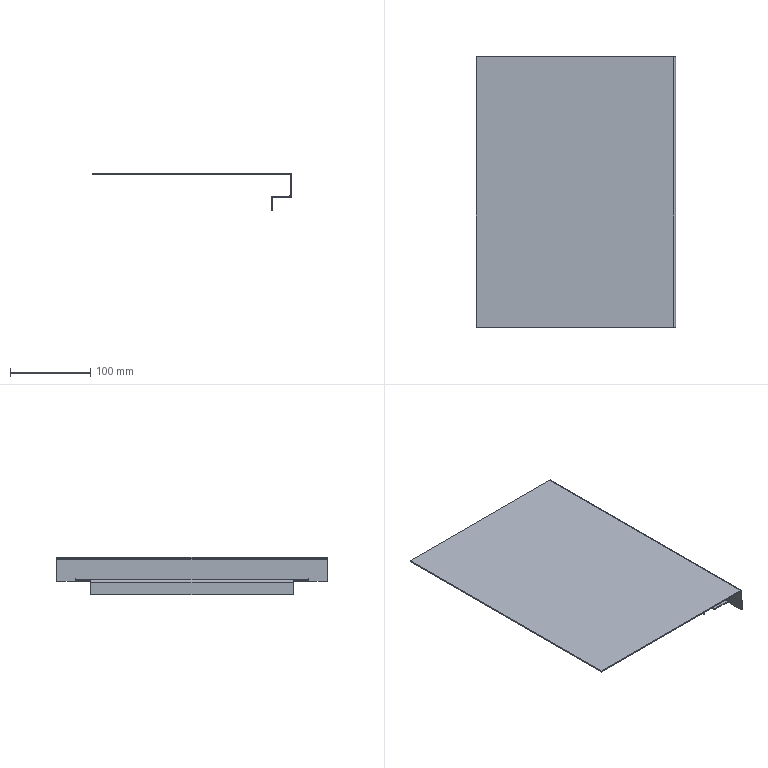Part | SolidWorks | features EdgeFlange 3, FlatPattern 1, SMBaseFlange 1, SheetMetal 1 | 1 solid | 46 faces | box 248.5 x 337 x 47 mm | volume 155691 mm3 | plane 40 | cylinder 6 | commonest cylinder face diameters 2 x3 5 x3
STEP:
#1=CARTESIAN_POINT('',(226.75,295.75,-30.));
#2=VERTEX_POINT('',#1);
#3=CARTESIAN_POINT('',(226.75,295.,-30.));
#4=VERTEX_POINT('',#3);
#5=CARTESIAN_POINT('',(226.75,295.75,-30.));
#6=DIRECTION('',(0.,-1.,0.));
#7=VECTOR('',#6,1000.);
#8=LINE('',#5,#7);
#9=EDGE_CURVE('',#2,#4,#8,.T.);
#10=ORIENTED_EDGE('',*,*,#9,.F.);
#11=CARTESIAN_POINT('',(223.5,295.75,-30.));
#12=VERTEX_POINT('',#11);
#13=CARTESIAN_POINT('',(223.5,295.75,-30.));
#14=DIRECTION('',(1.,0.,0.));
#15=VECTOR('',#14,1000.);
#16=LINE('',#13,#15);
#17=EDGE_CURVE('',#12,#2,#16,.T.);
#18=ORIENTED_EDGE('',*,*,#17,.F.);
#19=CARTESIAN_POINT('',(223.5,313.5,-30.));
#20=VERTEX_POINT('',#19);
#21=CARTESIAN_POINT('',(223.5,23.5,-30.));
#22=DIRECTION('',(0.,-1.,0.));
#23=VECTOR('',#22,1000.);
#24=LINE('',#21,#23);
#25=EDGE_CURVE('',#20,#12,#24,.T.);
#26=ORIENTED_EDGE('',*,*,#25,.F.);
#27=CARTESIAN_POINT('',(246.,313.5,-30.));
#28=VERTEX_POINT('',#27);
#29=CARTESIAN_POINT('',(223.5,313.5,-30.));
#30=DIRECTION('',(-1.,0.,0.));
#31=VECTOR('',#30,1000.);
#32=LINE('',#29,#31);
#33=EDGE_CURVE('',#28,#20,#32,.T.);
#34=ORIENTED_EDGE('',*,*,#33,.F.);
#35=CARTESIAN_POINT('',(246.,23.5,-30.));
#36=VERTEX_POINT('',#35);
#37=CARTESIAN_POINT('',(246.,0.,-30.));
#38=DIRECTION('',(0.,-1.,0.));
#39=VECTOR('',#38,1000.);
#40=LINE('',#37,#39);
#41=EDGE_CURVE('',#28,#36,#40,.T.);
#42=ORIENTED_EDGE('',*,*,#41,.T.);
#43=CARTESIAN_POINT('',(223.5,23.5,-30.));
#44=VERTEX_POINT('',#43);
#45=CARTESIAN_POINT('',(247.,23.5,-30.));
#46=DIRECTION('',(1.,0.,0.));
#47=VECTOR('',#46,1000.);
#48=LINE('',#45,#47);
#49=EDGE_CURVE('',#44,#36,#48,.T.);
#50=ORIENTED_EDGE('',*,*,#49,.F.);
#51=CARTESIAN_POINT('',(223.5,41.25,-30.));
#52=VERTEX_POINT('',#51);
#53=CARTESIAN_POINT('',(223.5,23.5,-30.));
#54=DIRECTION('',(0.,-1.,0.));
#55=VECTOR('',#54,1000.);
#56=LINE('',#53,#55);
#57=EDGE_CURVE('',#52,#44,#56,.T.);
#58=ORIENTED_EDGE('',*,*,#57,.F.);
#59=CARTESIAN_POINT('',(226.75,41.25,-30.));
#60=VERTEX_POINT('',#59);
#61=CARTESIAN_POINT('',(226.75,41.25,-30.));
#62=DIRECTION('',(-1.,0.,0.));
#63=VECTOR('',#62,1000.);
#64=LINE('',#61,#63);
#65=EDGE_CURVE('',#60,#52,#64,.T.);
#66=ORIENTED_EDGE('',*,*,#65,.F.);
#67=CARTESIAN_POINT('',(226.75,42.,-30.));
#68=VERTEX_POINT('',#67);
#69=CARTESIAN_POINT('',(226.75,42.,-30.));
#70=DIRECTION('',(0.,-1.,0.));
#71=VECTOR('',#70,1000.);
#72=LINE('',#69,#71);
#73=EDGE_CURVE('',#68,#60,#72,.T.);
#74=ORIENTED_EDGE('',*,*,#73,.F.);
#75=CARTESIAN_POINT('',(226.,42.,-30.));
#76=VERTEX_POINT('',#75);
#77=CARTESIAN_POINT('',(226.,42.,-30.));
#78=DIRECTION('',(1.,0.,0.));
#79=VECTOR('',#78,1000.);
#80=LINE('',#77,#79);
#81=EDGE_CURVE('',#76,#68,#80,.T.);
#82=ORIENTED_EDGE('',*,*,#81,.F.);
#83=CARTESIAN_POINT('',(226.,295.,-30.));
#84=VERTEX_POINT('',#83);
#85=CARTESIAN_POINT('',(226.,295.,-30.));
#86=DIRECTION('',(0.,-1.,0.));
#87=VECTOR('',#86,1000.);
#88=LINE('',#85,#87);
#89=EDGE_CURVE('',#84,#76,#88,.T.);
#90=ORIENTED_EDGE('',*,*,#89,.F.);
#91=CARTESIAN_POINT('',(226.75,295.,-30.));
#92=DIRECTION('',(-1.,0.,0.));
#93=VECTOR('',#92,1000.);
#94=LINE('',#91,#93);
#95=EDGE_CURVE('',#4,#84,#94,.T.);
#96=ORIENTED_EDGE('',*,*,#95,.F.);
#97=EDGE_LOOP('',(#10,#18,#26,#34,#42,#50,#58,#66,#74,#82,#90,#96));
#98=FACE_OUTER_BOUND('',#97,.T.);
#99=CARTESIAN_POINT('',(0.,0.,-30.));
#100=DIRECTION('',(0.,0.,-1.));
#101=DIRECTION('',(-1.,0.,0.));
#102=AXIS2_PLACEMENT_3D('',#99,#100,#101);
#103=PLANE('',#102);
#104=ADVANCED_FACE('',(#98),#103,.T.);
#105=CARTESIAN_POINT('',(226.75,295.75,-28.5));
#106=VERTEX_POINT('',#105);
#107=CARTESIAN_POINT('',(223.5,295.75,-28.5));
#108=VERTEX_POINT('',#107);
#109=CARTESIAN_POINT('',(0.,295.75,-28.5));
#110=DIRECTION('',(-1.,0.,0.));
#111=VECTOR('',#110,1000.);
#112=LINE('',#109,#111);
#113=EDGE_CURVE('',#106,#108,#112,.T.);
#114=ORIENTED_EDGE('',*,*,#113,.F.);
#115=CARTESIAN_POINT('',(226.75,295.,-28.5));
#116=VERTEX_POINT('',#115);
#117=CARTESIAN_POINT('',(226.75,0.,-28.5));
#118=DIRECTION('',(0.,1.,0.));
#119=VECTOR('',#118,1000.);
#120=LINE('',#117,#119);
#121=EDGE_CURVE('',#116,#106,#120,.T.);
#122=ORIENTED_EDGE('',*,*,#121,.F.);
#123=CARTESIAN_POINT('',(226.,295.,-28.5));
#124=VERTEX_POINT('',#123);
#125=CARTESIAN_POINT('',(0.,295.,-28.5));
#126=DIRECTION('',(1.,0.,0.));
#127=VECTOR('',#126,1000.);
#128=LINE('',#125,#127);
#129=EDGE_CURVE('',#124,#116,#128,.T.);
#130=ORIENTED_EDGE('',*,*,#129,.F.);
#131=CARTESIAN_POINT('',(226.,42.,-28.5));
#132=VERTEX_POINT('',#131);
#133=CARTESIAN_POINT('',(226.,295.,-28.5));
#134=DIRECTION('',(0.,-1.,0.));
#135=VECTOR('',#134,1000.);
#136=LINE('',#133,#135);
#137=EDGE_CURVE('',#124,#132,#136,.T.);
#138=ORIENTED_EDGE('',*,*,#137,.T.);
#139=CARTESIAN_POINT('',(226.75,42.,-28.5));
#140=VERTEX_POINT('',#139);
#141=CARTESIAN_POINT('',(0.,42.,-28.5));
#142=DIRECTION('',(-1.,0.,0.));
#143=VECTOR('',#142,1000.);
#144=LINE('',#141,#143);
#145=EDGE_CURVE('',#140,#132,#144,.T.);
#146=ORIENTED_EDGE('',*,*,#145,.F.);
#147=CARTESIAN_POINT('',(226.75,41.25,-28.5));
#148=VERTEX_POINT('',#147);
#149=CARTESIAN_POINT('',(226.75,0.,-28.5));
#150=DIRECTION('',(0.,1.,0.));
#151=VECTOR('',#150,1000.);
#152=LINE('',#149,#151);
#153=EDGE_CURVE('',#148,#140,#152,.T.);
#154=ORIENTED_EDGE('',*,*,#153,.F.);
#155=CARTESIAN_POINT('',(223.5,41.25,-28.5));
#156=VERTEX_POINT('',#155);
#157=CARTESIAN_POINT('',(0.,41.25,-28.5));
#158=DIRECTION('',(1.,0.,0.));
#159=VECTOR('',#158,1000.);
#160=LINE('',#157,#159);
#161=EDGE_CURVE('',#156,#148,#160,.T.);
#162=ORIENTED_EDGE('',*,*,#161,.F.);
#163=CARTESIAN_POINT('',(223.5,23.5,-28.5));
#164=VERTEX_POINT('',#163);
#165=CARTESIAN_POINT('',(223.5,0.,-28.5));
#166=DIRECTION('',(0.,-1.,0.));
#167=VECTOR('',#166,1000.);
#168=LINE('',#165,#167);
#169=EDGE_CURVE('',#156,#164,#168,.T.);
#170=ORIENTED_EDGE('',*,*,#169,.T.);
#171=CARTESIAN_POINT('',(246.,23.5,-28.5));
#172=VERTEX_POINT('',#171);
#173=CARTESIAN_POINT('',(0.,23.5,-28.5));
#174=DIRECTION('',(1.,0.,0.));
#175=VECTOR('',#174,1000.);
#176=LINE('',#173,#175);
#177=EDGE_CURVE('',#164,#172,#176,.T.);
#178=ORIENTED_EDGE('',*,*,#177,.T.);
#179=CARTESIAN_POINT('',(246.,313.5,-28.5));
#180=VERTEX_POINT('',#179);
#181=CARTESIAN_POINT('',(246.,313.5,-28.5));
#182=DIRECTION('',(0.,-1.,0.));
#183=VECTOR('',#182,1000.);
#184=LINE('',#181,#183);
#185=EDGE_CURVE('',#180,#172,#184,.T.);
#186=ORIENTED_EDGE('',*,*,#185,.F.);
#187=CARTESIAN_POINT('',(223.5,313.5,-28.5));
#188=VERTEX_POINT('',#187);
#189=CARTESIAN_POINT('',(0.,313.5,-28.5));
#190=DIRECTION('',(-1.,0.,0.));
#191=VECTOR('',#190,1000.);
#192=LINE('',#189,#191);
#193=EDGE_CURVE('',#180,#188,#192,.T.);
#194=ORIENTED_EDGE('',*,*,#193,.T.);
#195=CARTESIAN_POINT('',(223.5,0.,-28.5));
#196=DIRECTION('',(0.,-1.,0.));
#197=VECTOR('',#196,1000.);
#198=LINE('',#195,#197);
#199=EDGE_CURVE('',#188,#108,#198,.T.);
#200=ORIENTED_EDGE('',*,*,#199,.T.);
#201=EDGE_LOOP('',(#114,#122,#130,#138,#146,#154,#162,#170,#178,#186,#194,#200));
#202=FACE_OUTER_BOUND('',#201,.T.);
#203=CARTESIAN_POINT('',(0.,0.,-28.5));
#204=DIRECTION('',(0.,0.,-1.));
#205=DIRECTION('',(-1.,0.,0.));
#206=AXIS2_PLACEMENT_3D('',#203,#204,#205);
#207=PLANE('',#206);
#208=ADVANCED_FACE('',(#202),#207,.F.);
#209=ORIENTED_EDGE('',*,*,#25,.T.);
#210=CARTESIAN_POINT('',(223.5,295.75,-30.));
#211=DIRECTION('',(0.,0.,1.));
#212=VECTOR('',#211,1000.);
#213=LINE('',#210,#212);
#214=EDGE_CURVE('',#12,#108,#213,.T.);
#215=ORIENTED_EDGE('',*,*,#214,.T.);
#216=ORIENTED_EDGE('',*,*,#199,.F.);
#217=CARTESIAN_POINT('',(223.5,313.5,-30.));
#218=DIRECTION('',(0.,0.,1.));
#219=VECTOR('',#218,1000.);
#220=LINE('',#217,#219);
#221=EDGE_CURVE('',#20,#188,#220,.T.);
#222=ORIENTED_EDGE('',*,*,#221,.F.);
#223=EDGE_LOOP('',(#209,#215,#216,#222));
#224=FACE_OUTER_BOUND('',#223,.T.);
#225=CARTESIAN_POINT('',(223.5,23.5,-30.));
#226=DIRECTION('',(-1.,0.,0.));
#227=DIRECTION('',(0.,0.,1.));
#228=AXIS2_PLACEMENT_3D('',#225,#226,#227);
#229=PLANE('',#228);
#230=ADVANCED_FACE('',(#224),#229,.T.);
#231=ORIENTED_EDGE('',*,*,#169,.F.);
#232=CARTESIAN_POINT('',(223.5,41.25,-30.));
#233=DIRECTION('',(0.,0.,1.));
#234=VECTOR('',#233,1000.);
#235=LINE('',#232,#234);
#236=EDGE_CURVE('',#52,#156,#235,.T.);
#237=ORIENTED_EDGE('',*,*,#236,.F.);
#238=ORIENTED_EDGE('',*,*,#57,.T.);
#239=CARTESIAN_POINT('',(223.5,23.5,-30.));
#240=DIRECTION('',(0.,0.,1.));
#241=VECTOR('',#240,1000.);
#242=LINE('',#239,#241);
#243=EDGE_CURVE('',#44,#164,#242,.T.);
#244=ORIENTED_EDGE('',*,*,#243,.T.);
#245=EDGE_LOOP('',(#231,#237,#238,#244));
#246=FACE_OUTER_BOUND('',#245,.T.);
#247=CARTESIAN_POINT('',(223.5,23.5,-30.));
#248=DIRECTION('',(-1.,0.,0.));
#249=DIRECTION('',(0.,0.,1.));
#250=AXIS2_PLACEMENT_3D('',#247,#248,#249);
#251=PLANE('',#250);
#252=ADVANCED_FACE('',(#246),#251,.T.);
#253=CARTESIAN_POINT('',(248.5,22.75,-30.));
#254=VERTEX_POINT('',#253);
#255=CARTESIAN_POINT('',(248.5,0.,-30.));
#256=VERTEX_POINT('',#255);
#257=CARTESIAN_POINT('',(248.5,0.,-30.));
#258=DIRECTION('',(0.,-1.,0.));
#259=VECTOR('',#258,1000.);
#260=LINE('',#257,#259);
#261=EDGE_CURVE('',#254,#256,#260,.T.);
#262=ORIENTED_EDGE('',*,*,#261,.F.);
#263=CARTESIAN_POINT('',(248.5,22.75,-26.75));
#264=VERTEX_POINT('',#263);
#265=CARTESIAN_POINT('',(248.5,22.75,0.));
#266=DIRECTION('',(0.,0.,1.));
#267=VECTOR('',#266,1000.);
#268=LINE('',#265,#267);
#269=EDGE_CURVE('',#254,#264,#268,.T.);
#270=ORIENTED_EDGE('',*,*,#269,.T.);
#271=CARTESIAN_POINT('',(248.5,23.5,-26.75));
#272=VERTEX_POINT('',#271);
#273=CARTESIAN_POINT('',(248.5,0.,-26.75));
#274=DIRECTION('',(0.,1.,0.));
#275=VECTOR('',#274,1000.);
#276=LINE('',#273,#275);
#277=EDGE_CURVE('',#264,#272,#276,.T.);
#278=ORIENTED_EDGE('',*,*,#277,.T.);
#279=CARTESIAN_POINT('',(248.5,23.5,-27.5));
#280=VERTEX_POINT('',#279);
#281=CARTESIAN_POINT('',(248.5,23.5,0.));
#282=DIRECTION('',(0.,0.,-1.));
#283=VECTOR('',#282,1000.);
#284=LINE('',#281,#283);
#285=EDGE_CURVE('',#272,#280,#284,.T.);
#286=ORIENTED_EDGE('',*,*,#285,.T.);
#287=CARTESIAN_POINT('',(248.5,313.5,-27.5));
#288=VERTEX_POINT('',#287);
#289=CARTESIAN_POINT('',(248.5,23.5,-27.5));
#290=DIRECTION('',(0.,1.,0.));
#291=VECTOR('',#290,1000.);
#292=LINE('',#289,#291);
#293=EDGE_CURVE('',#280,#288,#292,.T.);
#294=ORIENTED_EDGE('',*,*,#293,.T.);
#295=CARTESIAN_POINT('',(248.5,313.5,-26.75));
#296=VERTEX_POINT('',#295);
#297=CARTESIAN_POINT('',(248.5,313.5,0.));
#298=DIRECTION('',(0.,0.,1.));
#299=VECTOR('',#298,1000.);
#300=LINE('',#297,#299);
#301=EDGE_CURVE('',#288,#296,#300,.T.);
#302=ORIENTED_EDGE('',*,*,#301,.T.);
#303=CARTESIAN_POINT('',(248.5,314.25,-26.75));
#304=VERTEX_POINT('',#303);
#305=CARTESIAN_POINT('',(248.5,0.,-26.75));
#306=DIRECTION('',(0.,1.,0.));
#307=VECTOR('',#306,1000.);
#308=LINE('',#305,#307);
#309=EDGE_CURVE('',#296,#304,#308,.T.);
#310=ORIENTED_EDGE('',*,*,#309,.T.);
#311=CARTESIAN_POINT('',(248.5,314.25,-30.));
#312=VERTEX_POINT('',#311);
#313=CARTESIAN_POINT('',(248.5,314.25,0.));
#314=DIRECTION('',(0.,0.,-1.));
#315=VECTOR('',#314,1000.);
#316=LINE('',#313,#315);
#317=EDGE_CURVE('',#304,#312,#316,.T.);
#318=ORIENTED_EDGE('',*,*,#317,.T.);
#319=CARTESIAN_POINT('',(248.5,337.,-30.));
#320=VERTEX_POINT('',#319);
#321=CARTESIAN_POINT('',(248.5,0.,-30.));
#322=DIRECTION('',(0.,-1.,0.));
#323=VECTOR('',#322,1000.);
#324=LINE('',#321,#323);
#325=EDGE_CURVE('',#320,#312,#324,.T.);
#326=ORIENTED_EDGE('',*,*,#325,.F.);
#327=CARTESIAN_POINT('',(248.5,337.,-2.5));
#328=VERTEX_POINT('',#327);
#329=CARTESIAN_POINT('',(248.5,337.,-30.));
#330=DIRECTION('',(0.,0.,-1.));
#331=VECTOR('',#330,1000.);
#332=LINE('',#329,#331);
#333=EDGE_CURVE('',#328,#320,#332,.T.);
#334=ORIENTED_EDGE('',*,*,#333,.F.);
#335=CARTESIAN_POINT('',(248.5,0.,-2.5));
#336=VERTEX_POINT('',#335);
#337=CARTESIAN_POINT('',(248.5,0.,-2.5));
#338=DIRECTION('',(0.,-1.,0.));
#339=VECTOR('',#338,1000.);
#340=LINE('',#337,#339);
#341=EDGE_CURVE('',#328,#336,#340,.T.);
#342=ORIENTED_EDGE('',*,*,#341,.T.);
#343=CARTESIAN_POINT('',(248.5,0.,-1.5));
#344=DIRECTION('',(0.,0.,1.));
#345=VECTOR('',#344,1000.);
#346=LINE('',#343,#345);
#347=EDGE_CURVE('',#256,#336,#346,.T.);
#348=ORIENTED_EDGE('',*,*,#347,.F.);
#349=EDGE_LOOP('',(#262,#270,#278,#286,#294,#302,#310,#318,#326,#334,#342,#348));
#350=FACE_OUTER_BOUND('',#349,.T.);
#351=CARTESIAN_POINT('',(248.5,0.,0.));
#352=DIRECTION('',(1.,0.,0.));
#353=DIRECTION('',(0.,0.,-1.));
#354=AXIS2_PLACEMENT_3D('',#351,#352,#353);
#355=PLANE('',#354);
#356=ADVANCED_FACE('',(#350),#355,.T.);
#357=CARTESIAN_POINT('',(247.,22.75,-30.));
#358=VERTEX_POINT('',#357);
#359=CARTESIAN_POINT('',(247.,22.75,-26.75));
#360=VERTEX_POINT('',#359);
#361=CARTESIAN_POINT('',(247.,22.75,-30.));
#362=DIRECTION('',(0.,0.,1.));
#363=VECTOR('',#362,1000.);
#364=LINE('',#361,#363);
#365=EDGE_CURVE('',#358,#360,#364,.T.);
#366=ORIENTED_EDGE('',*,*,#365,.F.);
#367=CARTESIAN_POINT('',(247.,0.,-30.));
#368=VERTEX_POINT('',#367);
#369=CARTESIAN_POINT('',(247.,0.,-30.));
#370=DIRECTION('',(0.,-1.,0.));
#371=VECTOR('',#370,1000.);
#372=LINE('',#369,#371);
#373=EDGE_CURVE('',#358,#368,#372,.T.);
#374=ORIENTED_EDGE('',*,*,#373,.T.);
#375=CARTESIAN_POINT('',(247.,0.,-2.5));
#376=VERTEX_POINT('',#375);
#377=CARTESIAN_POINT('',(247.,0.,0.));
#378=DIRECTION('',(0.,0.,1.));
#379=VECTOR('',#378,1000.);
#380=LINE('',#377,#379);
#381=EDGE_CURVE('',#368,#376,#380,.T.);
#382=ORIENTED_EDGE('',*,*,#381,.T.);
#383=CARTESIAN_POINT('',(247.,337.,-2.5));
#384=VERTEX_POINT('',#383);
#385=CARTESIAN_POINT('',(247.,337.,-2.5));
#386=DIRECTION('',(0.,-1.,0.));
#387=VECTOR('',#386,1000.);
#388=LINE('',#385,#387);
#389=EDGE_CURVE('',#384,#376,#388,.T.);
#390=ORIENTED_EDGE('',*,*,#389,.F.);
#391=CARTESIAN_POINT('',(247.,337.,-30.));
#392=VERTEX_POINT('',#391);
#393=CARTESIAN_POINT('',(247.,337.,0.));
#394=DIRECTION('',(0.,0.,-1.));
#395=VECTOR('',#394,1000.);
#396=LINE('',#393,#395);
#397=EDGE_CURVE('',#384,#392,#396,.T.);
#398=ORIENTED_EDGE('',*,*,#397,.T.);
#399=CARTESIAN_POINT('',(247.,314.25,-30.));
#400=VERTEX_POINT('',#399);
#401=CARTESIAN_POINT('',(247.,0.,-30.));
#402=DIRECTION('',(0.,-1.,0.));
#403=VECTOR('',#402,1000.);
#404=LINE('',#401,#403);
#405=EDGE_CURVE('',#392,#400,#404,.T.);
#406=ORIENTED_EDGE('',*,*,#405,.T.);
#407=CARTESIAN_POINT('',(247.,314.25,-26.75));
#408=VERTEX_POINT('',#407);
#409=CARTESIAN_POINT('',(247.,314.25,-26.75));
#410=DIRECTION('',(0.,0.,-1.));
#411=VECTOR('',#410,1000.);
#412=LINE('',#409,#411);
#413=EDGE_CURVE('',#408,#400,#412,.T.);
#414=ORIENTED_EDGE('',*,*,#413,.F.);
#415=CARTESIAN_POINT('',(247.,313.5,-26.75));
#416=VERTEX_POINT('',#415);
#417=CARTESIAN_POINT('',(247.,313.5,-26.75));
#418=DIRECTION('',(0.,1.,0.));
#419=VECTOR('',#418,1000.);
#420=LINE('',#417,#419);
#421=EDGE_CURVE('',#416,#408,#420,.T.);
#422=ORIENTED_EDGE('',*,*,#421,.F.);
#423=CARTESIAN_POINT('',(247.,313.5,-27.5));
#424=VERTEX_POINT('',#423);
#425=CARTESIAN_POINT('',(247.,313.5,-27.5));
#426=DIRECTION('',(0.,0.,1.));
#427=VECTOR('',#426,1000.);
#428=LINE('',#425,#427);
#429=EDGE_CURVE('',#424,#416,#428,.T.);
#430=ORIENTED_EDGE('',*,*,#429,.F.);
#431=CARTESIAN_POINT('',(247.,23.5,-27.5));
#432=VERTEX_POINT('',#431);
#433=CARTESIAN_POINT('',(247.,23.5,-27.5));
#434=DIRECTION('',(0.,1.,0.));
#435=VECTOR('',#434,1000.);
#436=LINE('',#433,#435);
#437=EDGE_CURVE('',#432,#424,#436,.T.);
#438=ORIENTED_EDGE('',*,*,#437,.F.);
#439=CARTESIAN_POINT('',(247.,23.5,-26.75));
#440=VERTEX_POINT('',#439);
#441=CARTESIAN_POINT('',(247.,23.5,-26.75));
#442=DIRECTION('',(0.,0.,-1.));
#443=VECTOR('',#442,1000.);
#444=LINE('',#441,#443);
#445=EDGE_CURVE('',#440,#432,#444,.T.);
#446=ORIENTED_EDGE('',*,*,#445,.F.);
#447=CARTESIAN_POINT('',(247.,22.75,-26.75));
#448=DIRECTION('',(0.,1.,0.));
#449=VECTOR('',#448,1000.);
#450=LINE('',#447,#449);
#451=EDGE_CURVE('',#360,#440,#450,.T.);
#452=ORIENTED_EDGE('',*,*,#451,.F.);
#453=EDGE_LOOP('',(#366,#374,#382,#390,#398,#406,#414,#422,#430,#438,#446,#452));
#454=FACE_OUTER_BOUND('',#453,.T.);
#455=CARTESIAN_POINT('',(247.,0.,0.));
#456=DIRECTION('',(1.,0.,0.));
#457=DIRECTION('',(0.,0.,-1.));
#458=AXIS2_PLACEMENT_3D('',#455,#456,#457);
#459=PLANE('',#458);
#460=ADVANCED_FACE('',(#454),#459,.F.);
#461=ORIENTED_EDGE('',*,*,#373,.F.);
#462=CARTESIAN_POINT('',(247.,22.75,-30.));
#463=DIRECTION('',(1.,0.,0.));
#464=VECTOR('',#463,1000.);
#465=LINE('',#462,#464);
#466=EDGE_CURVE('',#358,#254,#465,.T.);
#467=ORIENTED_EDGE('',*,*,#466,.T.);
#468=ORIENTED_EDGE('',*,*,#261,.T.);
#469=CARTESIAN_POINT('',(248.5,0.,-30.));
#470=DIRECTION('',(-1.,0.,0.));
#471=VECTOR('',#470,1000.);
#472=LINE('',#469,#471);
#473=EDGE_CURVE('',#256,#368,#472,.T.);
#474=ORIENTED_EDGE('',*,*,#473,.T.);
#475=EDGE_LOOP('',(#461,#467,#468,#474));
#476=FACE_OUTER_BOUND('',#475,.T.);
#477=CARTESIAN_POINT('',(248.5,0.,-30.));
#478=DIRECTION('',(0.,0.,-1.));
#479=DIRECTION('',(-1.,0.,0.));
#480=AXIS2_PLACEMENT_3D('',#477,#478,#479);
#481=PLANE('',#480);
#482=ADVANCED_FACE('',(#476),#481,.T.);
#483=ORIENTED_EDGE('',*,*,#325,.T.);
#484=CARTESIAN_POINT('',(247.,314.25,-30.));
#485=DIRECTION('',(1.,0.,0.));
#486=VECTOR('',#485,1000.);
#487=LINE('',#484,#486);
#488=EDGE_CURVE('',#400,#312,#487,.T.);
#489=ORIENTED_EDGE('',*,*,#488,.F.);
#490=ORIENTED_EDGE('',*,*,#405,.F.);
#491=CARTESIAN_POINT('',(248.5,337.,-30.));
#492=DIRECTION('',(-1.,0.,0.));
#493=VECTOR('',#492,1000.);
#494=LINE('',#491,#493);
#495=EDGE_CURVE('',#320,#392,#494,.T.);
#496=ORIENTED_EDGE('',*,*,#495,.F.);
#497=EDGE_LOOP('',(#483,#489,#490,#496));
#498=FACE_OUTER_BOUND('',#497,.T.);
#499=CARTESIAN_POINT('',(248.5,0.,-30.));
#500=DIRECTION('',(0.,0.,-1.));
#501=DIRECTION('',(-1.,0.,0.));
#502=AXIS2_PLACEMENT_3D('',#499,#500,#501);
#503=PLANE('',#502);
#504=ADVANCED_FACE('',(#498),#503,.T.);
#505=CARTESIAN_POINT('',(0.,0.,-1.5));
#506=VERTEX_POINT('',#505);
#507=CARTESIAN_POINT('',(246.,0.,-1.5));
#508=VERTEX_POINT('',#507);
#509=CARTESIAN_POINT('',(0.,0.,-1.5));
#510=DIRECTION('',(1.,0.,0.));
#511=VECTOR('',#510,1000.);
#512=LINE('',#509,#511);
#513=EDGE_CURVE('',#506,#508,#512,.T.);
#514=ORIENTED_EDGE('',*,*,#513,.T.);
#515=CARTESIAN_POINT('',(246.,0.,0.));
#516=VERTEX_POINT('',#515);
#517=CARTESIAN_POINT('',(246.,0.,-1.5));
#518=DIRECTION('',(0.,0.,1.));
#519=VECTOR('',#518,1000.);
#520=LINE('',#517,#519);
#521=EDGE_CURVE('',#508,#516,#520,.T.);
#522=ORIENTED_EDGE('',*,*,#521,.T.);
#523=CARTESIAN_POINT('',(0.,0.,0.));
#524=VERTEX_POINT('',#523);
#525=CARTESIAN_POINT('',(0.,0.,0.));
#526=DIRECTION('',(1.,0.,0.));
#527=VECTOR('',#526,1000.);
#528=LINE('',#525,#527);
#529=EDGE_CURVE('',#524,#516,#528,.T.);
#530=ORIENTED_EDGE('',*,*,#529,.F.);
#531=CARTESIAN_POINT('',(0.,0.,-1.5));
#532=DIRECTION('',(0.,0.,1.));
#533=VECTOR('',#532,1000.);
#534=LINE('',#531,#533);
#535=EDGE_CURVE('',#506,#524,#534,.T.);
#536=ORIENTED_EDGE('',*,*,#535,.F.);
#537=EDGE_LOOP('',(#514,#522,#530,#536));
#538=FACE_OUTER_BOUND('',#537,.T.);
#539=CARTESIAN_POINT('',(0.,0.,-1.5));
#540=DIRECTION('',(0.,-1.,0.));
#541=DIRECTION('',(0.,0.,-1.));
#542=AXIS2_PLACEMENT_3D('',#539,#540,#541);
#543=PLANE('',#542);
#544=ADVANCED_FACE('',(#538),#543,.T.);
#545=CARTESIAN_POINT('',(246.,337.,-1.5));
#546=VERTEX_POINT('',#545);
#547=CARTESIAN_POINT('',(0.,337.,-1.5));
#548=VERTEX_POINT('',#547);
#549=CARTESIAN_POINT('',(0.,337.,-1.5));
#550=DIRECTION('',(-1.,0.,0.));
#551=VECTOR('',#550,1000.);
#552=LINE('',#549,#551);
#553=EDGE_CURVE('',#546,#548,#552,.T.);
#554=ORIENTED_EDGE('',*,*,#553,.F.);
#555=CARTESIAN_POINT('',(246.,0.,-1.5));
#556=DIRECTION('',(0.,1.,0.));
#557=VECTOR('',#556,1000.);
#558=LINE('',#555,#557);
#559=EDGE_CURVE('',#508,#546,#558,.T.);
#560=ORIENTED_EDGE('',*,*,#559,.F.);
#561=ORIENTED_EDGE('',*,*,#513,.F.);
#562=CARTESIAN_POINT('',(0.,0.,-1.5));
#563=DIRECTION('',(0.,-1.,0.));
#564=VECTOR('',#563,1000.);
#565=LINE('',#562,#564);
#566=EDGE_CURVE('',#548,#506,#565,.T.);
#567=ORIENTED_EDGE('',*,*,#566,.F.);
#568=EDGE_LOOP('',(#554,#560,#561,#567));
#569=FACE_OUTER_BOUND('',#568,.T.);
#570=CARTESIAN_POINT('',(0.,0.,-1.5));
#571=DIRECTION('',(0.,0.,-1.));
#572=DIRECTION('',(-1.,0.,0.));
#573=AXIS2_PLACEMENT_3D('',#570,#571,#572);
#574=PLANE('',#573);
#575=ADVANCED_FACE('',(#569),#574,.T.);
#576=CARTESIAN_POINT('',(246.,337.,0.));
#577=VERTEX_POINT('',#576);
#578=CARTESIAN_POINT('',(246.,0.,0.));
#579=DIRECTION('',(0.,1.,0.));
#580=VECTOR('',#579,1000.);
#581=LINE('',#578,#580);
#582=EDGE_CURVE('',#516,#577,#581,.T.);
#583=ORIENTED_EDGE('',*,*,#582,.T.);
#584=CARTESIAN_POINT('',(0.,337.,0.));
#585=VERTEX_POINT('',#584);
#586=CARTESIAN_POINT('',(0.,337.,0.));
#587=DIRECTION('',(-1.,0.,0.));
#588=VECTOR('',#587,1000.);
#589=LINE('',#586,#588);
#590=EDGE_CURVE('',#577,#585,#589,.T.);
#591=ORIENTED_EDGE('',*,*,#590,.T.);
#592=CARTESIAN_POINT('',(0.,0.,0.));
#593=DIRECTION('',(0.,-1.,0.));
#594=VECTOR('',#593,1000.);
#595=LINE('',#592,#594);
#596=EDGE_CURVE('',#585,#524,#595,.T.);
#597=ORIENTED_EDGE('',*,*,#596,.T.);
#598=ORIENTED_EDGE('',*,*,#529,.T.);
#599=EDGE_LOOP('',(#583,#591,#597,#598));
#600=FACE_OUTER_BOUND('',#599,.T.);
#601=CARTESIAN_POINT('',(0.,0.,0.));
#602=DIRECTION('',(0.,0.,-1.));
#603=DIRECTION('',(-1.,0.,0.));
#604=AXIS2_PLACEMENT_3D('',#601,#602,#603);
#605=PLANE('',#604);
#606=ADVANCED_FACE('',(#600),#605,.F.);
#607=ORIENTED_EDGE('',*,*,#596,.F.);
#608=CARTESIAN_POINT('',(0.,337.,-1.5));
#609=DIRECTION('',(0.,0.,1.));
#610=VECTOR('',#609,1000.);
#611=LINE('',#608,#610);
#612=EDGE_CURVE('',#548,#585,#611,.T.);
#613=ORIENTED_EDGE('',*,*,#612,.F.);
#614=ORIENTED_EDGE('',*,*,#566,.T.);
#615=ORIENTED_EDGE('',*,*,#535,.T.);
#616=EDGE_LOOP('',(#607,#613,#614,#615));
#617=FACE_OUTER_BOUND('',#616,.T.);
#618=CARTESIAN_POINT('',(0.,0.,-1.5));
#619=DIRECTION('',(-1.,0.,0.));
#620=DIRECTION('',(0.,0.,1.));
#621=AXIS2_PLACEMENT_3D('',#618,#619,#620);
#622=PLANE('',#621);
#623=ADVANCED_FACE('',(#617),#622,.T.);
#624=CARTESIAN_POINT('',(246.,337.,-1.5));
#625=DIRECTION('',(0.,0.,1.));
#626=VECTOR('',#625,1000.);
#627=LINE('',#624,#626);
#628=EDGE_CURVE('',#546,#577,#627,.T.);
#629=ORIENTED_EDGE('',*,*,#628,.F.);
#630=ORIENTED_EDGE('',*,*,#553,.T.);
#631=ORIENTED_EDGE('',*,*,#612,.T.);
#632=ORIENTED_EDGE('',*,*,#590,.F.);
#633=EDGE_LOOP('',(#629,#630,#631,#632));
#634=FACE_OUTER_BOUND('',#633,.T.);
#635=CARTESIAN_POINT('',(0.,337.,-1.5));
#636=DIRECTION('',(0.,1.,0.));
#637=DIRECTION('',(0.,0.,1.));
#638=AXIS2_PLACEMENT_3D('',#635,#636,#637);
#639=PLANE('',#638);
#640=ADVANCED_FACE('',(#634),#639,.T.);
#641=CARTESIAN_POINT('',(248.5,337.,-2.5));
#642=DIRECTION('',(1.,0.,0.));
#643=VECTOR('',#642,1000.);
#644=LINE('',#641,#643);
#645=EDGE_CURVE('',#384,#328,#644,.T.);
#646=ORIENTED_EDGE('',*,*,#645,.F.);
#647=CARTESIAN_POINT('',(246.,337.,-2.5));
#648=DIRECTION('',(0.,1.,0.));
#649=DIRECTION('',(0.,0.,-1.));
#650=AXIS2_PLACEMENT_3D('',#647,#648,#649);
#651=CIRCLE('',#650,1.);
#652=EDGE_CURVE('',#546,#384,#651,.T.);
#653=ORIENTED_EDGE('',*,*,#652,.F.);
#654=ORIENTED_EDGE('',*,*,#628,.T.);
#655=CARTESIAN_POINT('',(246.,337.,-2.5));
#656=DIRECTION('',(0.,1.,0.));
#657=DIRECTION('',(0.,0.,-1.));
#658=AXIS2_PLACEMENT_3D('',#655,#656,#657);
#659=CIRCLE('',#658,2.5);
#660=EDGE_CURVE('',#577,#328,#659,.T.);
#661=ORIENTED_EDGE('',*,*,#660,.T.);
#662=EDGE_LOOP('',(#646,#653,#654,#661));
#663=FACE_OUTER_BOUND('',#662,.T.);
#664=CARTESIAN_POINT('',(246.,337.,-2.5));
#665=DIRECTION('',(0.,1.,0.));
#666=DIRECTION('',(0.,0.,1.));
#667=AXIS2_PLACEMENT_3D('',#664,#665,#666);
#668=PLANE('',#667);
#669=ADVANCED_FACE('',(#663),#668,.T.);
#670=CARTESIAN_POINT('',(246.,0.,-2.5));
#671=DIRECTION('',(0.,-1.,0.));
#672=DIRECTION('',(0.,0.,-1.));
#673=AXIS2_PLACEMENT_3D('',#670,#671,#672);
#674=CIRCLE('',#673,1.);
#675=EDGE_CURVE('',#376,#508,#674,.T.);
#676=ORIENTED_EDGE('',*,*,#675,.F.);
#677=CARTESIAN_POINT('',(247.,0.,-2.5));
#678=DIRECTION('',(1.,0.,0.));
#679=VECTOR('',#678,1000.);
#680=LINE('',#677,#679);
#681=EDGE_CURVE('',#376,#336,#680,.T.);
#682=ORIENTED_EDGE('',*,*,#681,.T.);
#683=CARTESIAN_POINT('',(246.,0.,-2.5));
#684=DIRECTION('',(0.,-1.,0.));
#685=DIRECTION('',(0.,0.,-1.));
#686=AXIS2_PLACEMENT_3D('',#683,#684,#685);
#687=CIRCLE('',#686,2.5);
#688=EDGE_CURVE('',#336,#516,#687,.T.);
#689=ORIENTED_EDGE('',*,*,#688,.T.);
#690=ORIENTED_EDGE('',*,*,#521,.F.);
#691=EDGE_LOOP('',(#676,#682,#689,#690));
#692=FACE_OUTER_BOUND('',#691,.T.);
#693=CARTESIAN_POINT('',(246.,0.,-2.5));
#694=DIRECTION('',(0.,1.,0.));
#695=DIRECTION('',(0.,0.,1.));
#696=AXIS2_PLACEMENT_3D('',#693,#694,#695);
#697=PLANE('',#696);
#698=ADVANCED_FACE('',(#692),#697,.F.);
#699=ORIENTED_EDGE('',*,*,#582,.F.);
#700=ORIENTED_EDGE('',*,*,#688,.F.);
#701=ORIENTED_EDGE('',*,*,#341,.F.);
#702=ORIENTED_EDGE('',*,*,#660,.F.);
#703=EDGE_LOOP('',(#699,#700,#701,#702));
#704=FACE_OUTER_BOUND('',#703,.T.);
#705=CARTESIAN_POINT('',(246.,0.,-2.5));
#706=DIRECTION('',(0.,-1.,0.));
#707=DIRECTION('',(1.,0.,0.));
#708=AXIS2_PLACEMENT_3D('',#705,#706,#707);
#709=CYLINDRICAL_SURFACE('',#708,2.5);
#710=ADVANCED_FACE('',(#704),#709,.T.);
#711=ORIENTED_EDGE('',*,*,#559,.T.);
#712=ORIENTED_EDGE('',*,*,#652,.T.);
#713=ORIENTED_EDGE('',*,*,#389,.T.);
#714=ORIENTED_EDGE('',*,*,#675,.T.);
#715=EDGE_LOOP('',(#711,#712,#713,#714));
#716=FACE_OUTER_BOUND('',#715,.T.);
#717=CARTESIAN_POINT('',(246.,0.,-2.5));
#718=DIRECTION('',(0.,-1.,0.));
#719=DIRECTION('',(1.,0.,0.));
#720=AXIS2_PLACEMENT_3D('',#717,#718,#719);
#721=CYLINDRICAL_SURFACE('',#720,1.);
#722=ADVANCED_FACE('',(#716),#721,.F.);
#723=ORIENTED_EDGE('',*,*,#347,.T.);
#724=ORIENTED_EDGE('',*,*,#681,.F.);
#725=ORIENTED_EDGE('',*,*,#381,.F.);
#726=ORIENTED_EDGE('',*,*,#473,.F.);
#727=EDGE_LOOP('',(#723,#724,#725,#726));
#728=FACE_OUTER_BOUND('',#727,.T.);
#729=CARTESIAN_POINT('',(248.5,0.,-1.5));
#730=DIRECTION('',(0.,-1.,0.));
#731=DIRECTION('',(0.,0.,-1.));
#732=AXIS2_PLACEMENT_3D('',#729,#730,#731);
#733=PLANE('',#732);
#734=ADVANCED_FACE('',(#728),#733,.T.);
#735=ORIENTED_EDGE('',*,*,#397,.F.);
#736=ORIENTED_EDGE('',*,*,#645,.T.);
#737=ORIENTED_EDGE('',*,*,#333,.T.);
#738=ORIENTED_EDGE('',*,*,#495,.T.);
#739=EDGE_LOOP('',(#735,#736,#737,#738));
#740=FACE_OUTER_BOUND('',#739,.T.);
#741=CARTESIAN_POINT('',(248.5,337.,-30.));
#742=DIRECTION('',(0.,1.,0.));
#743=DIRECTION('',(0.,0.,1.));
#744=AXIS2_PLACEMENT_3D('',#741,#742,#743);
#745=PLANE('',#744);
#746=ADVANCED_FACE('',(#740),#745,.T.);
#747=ORIENTED_EDGE('',*,*,#269,.F.);
#748=ORIENTED_EDGE('',*,*,#466,.F.);
#749=ORIENTED_EDGE('',*,*,#365,.T.);
#750=CARTESIAN_POINT('',(247.,22.75,-26.75));
#751=DIRECTION('',(1.,0.,0.));
#752=VECTOR('',#751,1000.);
#753=LINE('',#750,#752);
#754=EDGE_CURVE('',#360,#264,#753,.T.);
#755=ORIENTED_EDGE('',*,*,#754,.T.);
#756=EDGE_LOOP('',(#747,#748,#749,#755));
#757=FACE_OUTER_BOUND('',#756,.T.);
#758=CARTESIAN_POINT('',(247.,22.75,-30.));
#759=DIRECTION('',(0.,1.,0.));
#760=DIRECTION('',(0.,0.,1.));
#761=AXIS2_PLACEMENT_3D('',#758,#759,#760);
#762=PLANE('',#761);
#763=ADVANCED_FACE('',(#757),#762,.T.);
#764=ORIENTED_EDGE('',*,*,#277,.F.);
#765=ORIENTED_EDGE('',*,*,#754,.F.);
#766=ORIENTED_EDGE('',*,*,#451,.T.);
#767=CARTESIAN_POINT('',(247.,23.5,-26.75));
#768=DIRECTION('',(1.,0.,0.));
#769=VECTOR('',#768,1000.);
#770=LINE('',#767,#769);
#771=EDGE_CURVE('',#440,#272,#770,.T.);
#772=ORIENTED_EDGE('',*,*,#771,.T.);
#773=EDGE_LOOP('',(#764,#765,#766,#772));
#774=FACE_OUTER_BOUND('',#773,.T.);
#775=CARTESIAN_POINT('',(247.,22.75,-26.75));
#776=DIRECTION('',(0.,0.,-1.));
#777=DIRECTION('',(-1.,0.,0.));
#778=AXIS2_PLACEMENT_3D('',#775,#776,#777);
#779=PLANE('',#778);
#780=ADVANCED_FACE('',(#774),#779,.T.);
#781=ORIENTED_EDGE('',*,*,#285,.F.);
#782=ORIENTED_EDGE('',*,*,#771,.F.);
#783=ORIENTED_EDGE('',*,*,#445,.T.);
#784=CARTESIAN_POINT('',(247.,23.5,-27.5));
#785=DIRECTION('',(1.,0.,0.));
#786=VECTOR('',#785,1000.);
#787=LINE('',#784,#786);
#788=EDGE_CURVE('',#432,#280,#787,.T.);
#789=ORIENTED_EDGE('',*,*,#788,.T.);
#790=EDGE_LOOP('',(#781,#782,#783,#789));
#791=FACE_OUTER_BOUND('',#790,.T.);
#792=CARTESIAN_POINT('',(247.,23.5,-26.75));
#793=DIRECTION('',(0.,-1.,0.));
#794=DIRECTION('',(0.,0.,-1.));
#795=AXIS2_PLACEMENT_3D('',#792,#793,#794);
#796=PLANE('',#795);
#797=ADVANCED_FACE('',(#791),#796,.T.);
#798=ORIENTED_EDGE('',*,*,#301,.F.);
#799=CARTESIAN_POINT('',(247.,313.5,-27.5));
#800=DIRECTION('',(1.,0.,0.));
#801=VECTOR('',#800,1000.);
#802=LINE('',#799,#801);
#803=EDGE_CURVE('',#424,#288,#802,.T.);
#804=ORIENTED_EDGE('',*,*,#803,.F.);
#805=ORIENTED_EDGE('',*,*,#429,.T.);
#806=CARTESIAN_POINT('',(247.,313.5,-26.75));
#807=DIRECTION('',(1.,0.,0.));
#808=VECTOR('',#807,1000.);
#809=LINE('',#806,#808);
#810=EDGE_CURVE('',#416,#296,#809,.T.);
#811=ORIENTED_EDGE('',*,*,#810,.T.);
#812=EDGE_LOOP('',(#798,#804,#805,#811));
#813=FACE_OUTER_BOUND('',#812,.T.);
#814=CARTESIAN_POINT('',(247.,313.5,-27.5));
#815=DIRECTION('',(0.,1.,0.));
#816=DIRECTION('',(0.,0.,1.));
#817=AXIS2_PLACEMENT_3D('',#814,#815,#816);
#818=PLANE('',#817);
#819=ADVANCED_FACE('',(#813),#818,.T.);
#820=ORIENTED_EDGE('',*,*,#309,.F.);
#821=ORIENTED_EDGE('',*,*,#810,.F.);
#822=ORIENTED_EDGE('',*,*,#421,.T.);
#823=CARTESIAN_POINT('',(247.,314.25,-26.75));
#824=DIRECTION('',(1.,0.,0.));
#825=VECTOR('',#824,1000.);
#826=LINE('',#823,#825);
#827=EDGE_CURVE('',#408,#304,#826,.T.);
#828=ORIENTED_EDGE('',*,*,#827,.T.);
#829=EDGE_LOOP('',(#820,#821,#822,#828));
#830=FACE_OUTER_BOUND('',#829,.T.);
#831=CARTESIAN_POINT('',(247.,313.5,-26.75));
#832=DIRECTION('',(0.,0.,-1.));
#833=DIRECTION('',(-1.,0.,0.));
#834=AXIS2_PLACEMENT_3D('',#831,#832,#833);
#835=PLANE('',#834);
#836=ADVANCED_FACE('',(#830),#835,.T.);
#837=ORIENTED_EDGE('',*,*,#317,.F.);
#838=ORIENTED_EDGE('',*,*,#827,.F.);
#839=ORIENTED_EDGE('',*,*,#413,.T.);
#840=ORIENTED_EDGE('',*,*,#488,.T.);
#841=EDGE_LOOP('',(#837,#838,#839,#840));
#842=FACE_OUTER_BOUND('',#841,.T.);
#843=CARTESIAN_POINT('',(247.,314.25,-26.75));
#844=DIRECTION('',(0.,-1.,0.));
#845=DIRECTION('',(0.,0.,-1.));
#846=AXIS2_PLACEMENT_3D('',#843,#844,#845);
#847=PLANE('',#846);
#848=ADVANCED_FACE('',(#842),#847,.T.);
#849=CARTESIAN_POINT('',(246.,313.5,-30.));
#850=DIRECTION('',(0.,0.,-1.));
#851=VECTOR('',#850,1000.);
#852=LINE('',#849,#851);
#853=EDGE_CURVE('',#180,#28,#852,.T.);
#854=ORIENTED_EDGE('',*,*,#853,.F.);
#855=CARTESIAN_POINT('',(246.,313.5,-27.5));
#856=DIRECTION('',(0.,1.,0.));
#857=DIRECTION('',(0.,0.,-1.));
#858=AXIS2_PLACEMENT_3D('',#855,#856,#857);
#859=CIRCLE('',#858,1.);
#860=EDGE_CURVE('',#424,#180,#859,.T.);
#861=ORIENTED_EDGE('',*,*,#860,.F.);
#862=ORIENTED_EDGE('',*,*,#803,.T.);
#863=CARTESIAN_POINT('',(246.,313.5,-27.5));
#864=DIRECTION('',(0.,1.,0.));
#865=DIRECTION('',(0.,0.,-1.));
#866=AXIS2_PLACEMENT_3D('',#863,#864,#865);
#867=CIRCLE('',#866,2.5);
#868=EDGE_CURVE('',#288,#28,#867,.T.);
#869=ORIENTED_EDGE('',*,*,#868,.T.);
#870=EDGE_LOOP('',(#854,#861,#862,#869));
#871=FACE_OUTER_BOUND('',#870,.T.);
#872=CARTESIAN_POINT('',(246.,313.5,-27.5));
#873=DIRECTION('',(0.,1.,0.));
#874=DIRECTION('',(0.,0.,1.));
#875=AXIS2_PLACEMENT_3D('',#872,#873,#874);
#876=PLANE('',#875);
#877=ADVANCED_FACE('',(#871),#876,.T.);
#878=CARTESIAN_POINT('',(246.,23.5,-27.5));
#879=DIRECTION('',(0.,-1.,0.));
#880=DIRECTION('',(0.,0.,-1.));
#881=AXIS2_PLACEMENT_3D('',#878,#879,#880);
#882=CIRCLE('',#881,1.);
#883=EDGE_CURVE('',#172,#432,#882,.T.);
#884=ORIENTED_EDGE('',*,*,#883,.F.);
#885=CARTESIAN_POINT('',(246.,23.5,-28.5));
#886=DIRECTION('',(0.,0.,-1.));
#887=VECTOR('',#886,1000.);
#888=LINE('',#885,#887);
#889=EDGE_CURVE('',#172,#36,#888,.T.);
#890=ORIENTED_EDGE('',*,*,#889,.T.);
#891=CARTESIAN_POINT('',(246.,23.5,-27.5));
#892=DIRECTION('',(0.,-1.,0.));
#893=DIRECTION('',(0.,0.,-1.));
#894=AXIS2_PLACEMENT_3D('',#891,#892,#893);
#895=CIRCLE('',#894,2.5);
#896=EDGE_CURVE('',#36,#280,#895,.T.);
#897=ORIENTED_EDGE('',*,*,#896,.T.);
#898=ORIENTED_EDGE('',*,*,#788,.F.);
#899=EDGE_LOOP('',(#884,#890,#897,#898));
#900=FACE_OUTER_BOUND('',#899,.T.);
#901=CARTESIAN_POINT('',(246.,23.5,-27.5));
#902=DIRECTION('',(0.,1.,0.));
#903=DIRECTION('',(0.,0.,1.));
#904=AXIS2_PLACEMENT_3D('',#901,#902,#903);
#905=PLANE('',#904);
#906=ADVANCED_FACE('',(#900),#905,.F.);
#907=ORIENTED_EDGE('',*,*,#293,.F.);
#908=ORIENTED_EDGE('',*,*,#896,.F.);
#909=ORIENTED_EDGE('',*,*,#41,.F.);
#910=ORIENTED_EDGE('',*,*,#868,.F.);
#911=EDGE_LOOP('',(#907,#908,#909,#910));
#912=FACE_OUTER_BOUND('',#911,.T.);
#913=CARTESIAN_POINT('',(246.,23.5,-27.5));
#914=DIRECTION('',(0.,-1.,0.));
#915=DIRECTION('',(0.,0.,-1.));
#916=AXIS2_PLACEMENT_3D('',#913,#914,#915);
#917=CYLINDRICAL_SURFACE('',#916,2.5);
#918=ADVANCED_FACE('',(#912),#917,.T.);
#919=ORIENTED_EDGE('',*,*,#437,.T.);
#920=ORIENTED_EDGE('',*,*,#860,.T.);
#921=ORIENTED_EDGE('',*,*,#185,.T.);
#922=ORIENTED_EDGE('',*,*,#883,.T.);
#923=EDGE_LOOP('',(#919,#920,#921,#922));
#924=FACE_OUTER_BOUND('',#923,.T.);
#925=CARTESIAN_POINT('',(246.,23.5,-27.5));
#926=DIRECTION('',(0.,-1.,0.));
#927=DIRECTION('',(0.,0.,-1.));
#928=AXIS2_PLACEMENT_3D('',#925,#926,#927);
#929=CYLINDRICAL_SURFACE('',#928,1.);
#930=ADVANCED_FACE('',(#924),#929,.F.);
#931=ORIENTED_EDGE('',*,*,#49,.T.);
#932=ORIENTED_EDGE('',*,*,#889,.F.);
#933=ORIENTED_EDGE('',*,*,#177,.F.);
#934=ORIENTED_EDGE('',*,*,#243,.F.);
#935=EDGE_LOOP('',(#931,#932,#933,#934));
#936=FACE_OUTER_BOUND('',#935,.T.);
#937=CARTESIAN_POINT('',(247.,23.5,-30.));
#938=DIRECTION('',(0.,-1.,0.));
#939=DIRECTION('',(1.,0.,0.));
#940=AXIS2_PLACEMENT_3D('',#937,#938,#939);
#941=PLANE('',#940);
#942=ADVANCED_FACE('',(#936),#941,.T.);
#943=ORIENTED_EDGE('',*,*,#193,.F.);
#944=ORIENTED_EDGE('',*,*,#853,.T.);
#945=ORIENTED_EDGE('',*,*,#33,.T.);
#946=ORIENTED_EDGE('',*,*,#221,.T.);
#947=EDGE_LOOP('',(#943,#944,#945,#946));
#948=FACE_OUTER_BOUND('',#947,.T.);
#949=CARTESIAN_POINT('',(223.5,313.5,-30.));
#950=DIRECTION('',(0.,1.,0.));
#951=DIRECTION('',(0.,0.,1.));
#952=AXIS2_PLACEMENT_3D('',#949,#950,#951);
#953=PLANE('',#952);
#954=ADVANCED_FACE('',(#948),#953,.T.);
#955=CARTESIAN_POINT('',(226.75,295.,-30.));
#956=DIRECTION('',(0.,0.,1.));
#957=VECTOR('',#956,1000.);
#958=LINE('',#955,#957);
#959=EDGE_CURVE('',#4,#116,#958,.T.);
#960=ORIENTED_EDGE('',*,*,#959,.T.);
#961=ORIENTED_EDGE('',*,*,#121,.T.);
#962=CARTESIAN_POINT('',(226.75,295.75,-30.));
#963=DIRECTION('',(0.,0.,1.));
#964=VECTOR('',#963,1000.);
#965=LINE('',#962,#964);
#966=EDGE_CURVE('',#2,#106,#965,.T.);
#967=ORIENTED_EDGE('',*,*,#966,.F.);
#968=ORIENTED_EDGE('',*,*,#9,.T.);
#969=EDGE_LOOP('',(#960,#961,#967,#968));
#970=FACE_OUTER_BOUND('',#969,.T.);
#971=CARTESIAN_POINT('',(226.75,295.75,-30.));
#972=DIRECTION('',(-1.,0.,0.));
#973=DIRECTION('',(0.,0.,1.));
#974=AXIS2_PLACEMENT_3D('',#971,#972,#973);
#975=PLANE('',#974);
#976=ADVANCED_FACE('',(#970),#975,.T.);
#977=CARTESIAN_POINT('',(226.,295.,-30.));
#978=DIRECTION('',(0.,0.,1.));
#979=VECTOR('',#978,1000.);
#980=LINE('',#977,#979);
#981=EDGE_CURVE('',#84,#124,#980,.T.);
#982=ORIENTED_EDGE('',*,*,#981,.T.);
#983=ORIENTED_EDGE('',*,*,#129,.T.);
#984=ORIENTED_EDGE('',*,*,#959,.F.);
#985=ORIENTED_EDGE('',*,*,#95,.T.);
#986=EDGE_LOOP('',(#982,#983,#984,#985));
#987=FACE_OUTER_BOUND('',#986,.T.);
#988=CARTESIAN_POINT('',(226.75,295.,-30.));
#989=DIRECTION('',(0.,1.,0.));
#990=DIRECTION('',(0.,0.,1.));
#991=AXIS2_PLACEMENT_3D('',#988,#989,#990);
#992=PLANE('',#991);
#993=ADVANCED_FACE('',(#987),#992,.T.);
#994=CARTESIAN_POINT('',(226.75,42.,-30.));
#995=DIRECTION('',(0.,0.,1.));
#996=VECTOR('',#995,1000.);
#997=LINE('',#994,#996);
#998=EDGE_CURVE('',#68,#140,#997,.T.);
#999=ORIENTED_EDGE('',*,*,#998,.T.);
#1000=ORIENTED_EDGE('',*,*,#145,.T.);
#1001=CARTESIAN_POINT('',(226.,42.,-30.));
#1002=DIRECTION('',(0.,0.,1.));
#1003=VECTOR('',#1002,1000.);
#1004=LINE('',#1001,#1003);
#1005=EDGE_CURVE('',#76,#132,#1004,.T.);
#1006=ORIENTED_EDGE('',*,*,#1005,.F.);
#1007=ORIENTED_EDGE('',*,*,#81,.T.);
#1008=EDGE_LOOP('',(#999,#1000,#1006,#1007));
#1009=FACE_OUTER_BOUND('',#1008,.T.);
#1010=CARTESIAN_POINT('',(226.,42.,-30.));
#1011=DIRECTION('',(0.,-1.,0.));
#1012=DIRECTION('',(0.,0.,-1.));
#1013=AXIS2_PLACEMENT_3D('',#1010,#1011,#1012);
#1014=PLANE('',#1013);
#1015=ADVANCED_FACE('',(#1009),#1014,.T.);
#1016=CARTESIAN_POINT('',(226.75,41.25,-30.));
#1017=DIRECTION('',(0.,0.,1.));
#1018=VECTOR('',#1017,1000.);
#1019=LINE('',#1016,#1018);
#1020=EDGE_CURVE('',#60,#148,#1019,.T.);
#1021=ORIENTED_EDGE('',*,*,#1020,.T.);
#1022=ORIENTED_EDGE('',*,*,#153,.T.);
#1023=ORIENTED_EDGE('',*,*,#998,.F.);
#1024=ORIENTED_EDGE('',*,*,#73,.T.);
#1025=EDGE_LOOP('',(#1021,#1022,#1023,#1024));
#1026=FACE_OUTER_BOUND('',#1025,.T.);
#1027=CARTESIAN_POINT('',(226.75,42.,-30.));
#1028=DIRECTION('',(-1.,0.,0.));
#1029=DIRECTION('',(0.,0.,1.));
#1030=AXIS2_PLACEMENT_3D('',#1027,#1028,#1029);
#1031=PLANE('',#1030);
#1032=ADVANCED_FACE('',(#1026),#1031,.T.);
#1033=ORIENTED_EDGE('',*,*,#966,.T.);
#1034=ORIENTED_EDGE('',*,*,#113,.T.);
#1035=ORIENTED_EDGE('',*,*,#214,.F.);
#1036=ORIENTED_EDGE('',*,*,#17,.T.);
#1037=EDGE_LOOP('',(#1033,#1034,#1035,#1036));
#1038=FACE_OUTER_BOUND('',#1037,.T.);
#1039=CARTESIAN_POINT('',(223.5,295.75,-30.));
#1040=DIRECTION('',(0.,-1.,0.));
#1041=DIRECTION('',(0.,0.,-1.));
#1042=AXIS2_PLACEMENT_3D('',#1039,#1040,#1041);
#1043=PLANE('',#1042);
#1044=ADVANCED_FACE('',(#1038),#1043,.T.);
#1045=ORIENTED_EDGE('',*,*,#236,.T.);
#1046=ORIENTED_EDGE('',*,*,#161,.T.);
#1047=ORIENTED_EDGE('',*,*,#1020,.F.);
#1048=ORIENTED_EDGE('',*,*,#65,.T.);
#1049=EDGE_LOOP('',(#1045,#1046,#1047,#1048));
#1050=FACE_OUTER_BOUND('',#1049,.T.);
#1051=CARTESIAN_POINT('',(226.75,41.25,-30.));
#1052=DIRECTION('',(0.,1.,0.));
#1053=DIRECTION('',(0.,0.,1.));
#1054=AXIS2_PLACEMENT_3D('',#1051,#1052,#1053);
#1055=PLANE('',#1054);
#1056=ADVANCED_FACE('',(#1050),#1055,.T.);
#1057=CARTESIAN_POINT('',(225.,42.,-31.));
#1058=VERTEX_POINT('',#1057);
#1059=CARTESIAN_POINT('',(223.5,42.,-31.));
#1060=VERTEX_POINT('',#1059);
#1061=CARTESIAN_POINT('',(223.5,42.,-31.));
#1062=DIRECTION('',(-1.,0.,0.));
#1063=VECTOR('',#1062,1000.);
#1064=LINE('',#1061,#1063);
#1065=EDGE_CURVE('',#1058,#1060,#1064,.T.);
#1066=ORIENTED_EDGE('',*,*,#1065,.F.);
#1067=CARTESIAN_POINT('',(226.,42.,-31.));
#1068=DIRECTION('',(0.,-1.,0.));
#1069=DIRECTION('',(0.,0.,1.));
#1070=AXIS2_PLACEMENT_3D('',#1067,#1068,#1069);
#1071=CIRCLE('',#1070,1.);
#1072=EDGE_CURVE('',#76,#1058,#1071,.T.);
#1073=ORIENTED_EDGE('',*,*,#1072,.F.);
#1074=ORIENTED_EDGE('',*,*,#1005,.T.);
#1075=CARTESIAN_POINT('',(226.,42.,-31.));
#1076=DIRECTION('',(0.,-1.,0.));
#1077=DIRECTION('',(0.,0.,1.));
#1078=AXIS2_PLACEMENT_3D('',#1075,#1076,#1077);
#1079=CIRCLE('',#1078,2.5);
#1080=EDGE_CURVE('',#132,#1060,#1079,.T.);
#1081=ORIENTED_EDGE('',*,*,#1080,.T.);
#1082=EDGE_LOOP('',(#1066,#1073,#1074,#1081));
#1083=FACE_OUTER_BOUND('',#1082,.T.);
#1084=CARTESIAN_POINT('',(226.,42.,-31.));
#1085=DIRECTION('',(0.,-1.,0.));
#1086=DIRECTION('',(0.,0.,-1.));
#1087=AXIS2_PLACEMENT_3D('',#1084,#1085,#1086);
#1088=PLANE('',#1087);
#1089=ADVANCED_FACE('',(#1083),#1088,.T.);
#1090=CARTESIAN_POINT('',(225.,295.,-31.));
#1091=VERTEX_POINT('',#1090);
#1092=CARTESIAN_POINT('',(226.,295.,-31.));
#1093=DIRECTION('',(0.,1.,0.));
#1094=DIRECTION('',(0.,0.,1.));
#1095=AXIS2_PLACEMENT_3D('',#1092,#1093,#1094);
#1096=CIRCLE('',#1095,1.);
#1097=EDGE_CURVE('',#1091,#84,#1096,.T.);
#1098=ORIENTED_EDGE('',*,*,#1097,.F.);
#1099=CARTESIAN_POINT('',(223.5,295.,-31.));
#1100=VERTEX_POINT('',#1099);
#1101=CARTESIAN_POINT('',(225.,295.,-31.));
#1102=DIRECTION('',(-1.,0.,0.));
#1103=VECTOR('',#1102,1000.);
#1104=LINE('',#1101,#1103);
#1105=EDGE_CURVE('',#1091,#1100,#1104,.T.);
#1106=ORIENTED_EDGE('',*,*,#1105,.T.);
#1107=CARTESIAN_POINT('',(226.,295.,-31.));
#1108=DIRECTION('',(0.,1.,0.));
#1109=DIRECTION('',(0.,0.,1.));
#1110=AXIS2_PLACEMENT_3D('',#1107,#1108,#1109);
#1111=CIRCLE('',#1110,2.5);
#1112=EDGE_CURVE('',#1100,#124,#1111,.T.);
#1113=ORIENTED_EDGE('',*,*,#1112,.T.);
#1114=ORIENTED_EDGE('',*,*,#981,.F.);
#1115=EDGE_LOOP('',(#1098,#1106,#1113,#1114));
#1116=FACE_OUTER_BOUND('',#1115,.T.);
#1117=CARTESIAN_POINT('',(226.,295.,-31.));
#1118=DIRECTION('',(0.,-1.,0.));
#1119=DIRECTION('',(0.,0.,-1.));
#1120=AXIS2_PLACEMENT_3D('',#1117,#1118,#1119);
#1121=PLANE('',#1120);
#1122=ADVANCED_FACE('',(#1116),#1121,.F.);
#1123=ORIENTED_EDGE('',*,*,#137,.F.);
#1124=ORIENTED_EDGE('',*,*,#1112,.F.);
#1125=CARTESIAN_POINT('',(223.5,0.,-31.));
#1126=DIRECTION('',(0.,1.,0.));
#1127=VECTOR('',#1126,1000.);
#1128=LINE('',#1125,#1127);
#1129=EDGE_CURVE('',#1060,#1100,#1128,.T.);
#1130=ORIENTED_EDGE('',*,*,#1129,.F.);
#1131=ORIENTED_EDGE('',*,*,#1080,.F.);
#1132=EDGE_LOOP('',(#1123,#1124,#1130,#1131));
#1133=FACE_OUTER_BOUND('',#1132,.T.);
#1134=CARTESIAN_POINT('',(226.,295.,-31.));
#1135=DIRECTION('',(0.,1.,0.));
#1136=DIRECTION('',(-1.,0.,0.));
#1137=AXIS2_PLACEMENT_3D('',#1134,#1135,#1136);
#1138=CYLINDRICAL_SURFACE('',#1137,2.5);
#1139=ADVANCED_FACE('',(#1133),#1138,.T.);
#1140=ORIENTED_EDGE('',*,*,#89,.T.);
#1141=ORIENTED_EDGE('',*,*,#1072,.T.);
#1142=CARTESIAN_POINT('',(225.,42.,-31.));
#1143=DIRECTION('',(0.,1.,0.));
#1144=VECTOR('',#1143,1000.);
#1145=LINE('',#1142,#1144);
#1146=EDGE_CURVE('',#1058,#1091,#1145,.T.);
#1147=ORIENTED_EDGE('',*,*,#1146,.T.);
#1148=ORIENTED_EDGE('',*,*,#1097,.T.);
#1149=EDGE_LOOP('',(#1140,#1141,#1147,#1148));
#1150=FACE_OUTER_BOUND('',#1149,.T.);
#1151=CARTESIAN_POINT('',(226.,295.,-31.));
#1152=DIRECTION('',(0.,1.,0.));
#1153=DIRECTION('',(-1.,0.,0.));
#1154=AXIS2_PLACEMENT_3D('',#1151,#1152,#1153);
#1155=CYLINDRICAL_SURFACE('',#1154,1.);
#1156=ADVANCED_FACE('',(#1150),#1155,.F.);
#1157=CARTESIAN_POINT('',(223.5,295.,-47.));
#1158=VERTEX_POINT('',#1157);
#1159=CARTESIAN_POINT('',(223.5,295.,-30.));
#1160=DIRECTION('',(0.,0.,1.));
#1161=VECTOR('',#1160,1000.);
#1162=LINE('',#1159,#1161);
#1163=EDGE_CURVE('',#1158,#1100,#1162,.T.);
#1164=ORIENTED_EDGE('',*,*,#1163,.T.);
#1165=ORIENTED_EDGE('',*,*,#1105,.F.);
#1166=CARTESIAN_POINT('',(225.,295.,-47.));
#1167=VERTEX_POINT('',#1166);
#1168=CARTESIAN_POINT('',(225.,295.,0.));
#1169=DIRECTION('',(0.,0.,1.));
#1170=VECTOR('',#1169,1000.);
#1171=LINE('',#1168,#1170);
#1172=EDGE_CURVE('',#1167,#1091,#1171,.T.);
#1173=ORIENTED_EDGE('',*,*,#1172,.F.);
#1174=CARTESIAN_POINT('',(223.5,295.,-47.));
#1175=DIRECTION('',(1.,0.,0.));
#1176=VECTOR('',#1175,1000.);
#1177=LINE('',#1174,#1176);
#1178=EDGE_CURVE('',#1158,#1167,#1177,.T.);
#1179=ORIENTED_EDGE('',*,*,#1178,.F.);
#1180=EDGE_LOOP('',(#1164,#1165,#1173,#1179));
#1181=FACE_OUTER_BOUND('',#1180,.T.);
#1182=CARTESIAN_POINT('',(223.5,295.,-30.));
#1183=DIRECTION('',(0.,1.,0.));
#1184=DIRECTION('',(0.,0.,1.));
#1185=AXIS2_PLACEMENT_3D('',#1182,#1183,#1184);
#1186=PLANE('',#1185);
#1187=ADVANCED_FACE('',(#1181),#1186,.T.);
#1188=CARTESIAN_POINT('',(225.,42.,-47.));
#1189=VERTEX_POINT('',#1188);
#1190=CARTESIAN_POINT('',(225.,42.,0.));
#1191=DIRECTION('',(0.,0.,-1.));
#1192=VECTOR('',#1191,1000.);
#1193=LINE('',#1190,#1192);
#1194=EDGE_CURVE('',#1058,#1189,#1193,.T.);
#1195=ORIENTED_EDGE('',*,*,#1194,.F.);
#1196=ORIENTED_EDGE('',*,*,#1065,.T.);
#1197=CARTESIAN_POINT('',(223.5,42.,-47.));
#1198=VERTEX_POINT('',#1197);
#1199=CARTESIAN_POINT('',(223.5,42.,-47.));
#1200=DIRECTION('',(0.,0.,-1.));
#1201=VECTOR('',#1200,1000.);
#1202=LINE('',#1199,#1201);
#1203=EDGE_CURVE('',#1060,#1198,#1202,.T.);
#1204=ORIENTED_EDGE('',*,*,#1203,.T.);
#1205=CARTESIAN_POINT('',(223.5,42.,-47.));
#1206=DIRECTION('',(1.,0.,0.));
#1207=VECTOR('',#1206,1000.);
#1208=LINE('',#1205,#1207);
#1209=EDGE_CURVE('',#1198,#1189,#1208,.T.);
#1210=ORIENTED_EDGE('',*,*,#1209,.T.);
#1211=EDGE_LOOP('',(#1195,#1196,#1204,#1210));
#1212=FACE_OUTER_BOUND('',#1211,.T.);
#1213=CARTESIAN_POINT('',(223.5,42.,-47.));
#1214=DIRECTION('',(0.,-1.,0.));
#1215=DIRECTION('',(0.,0.,-1.));
#1216=AXIS2_PLACEMENT_3D('',#1213,#1214,#1215);
#1217=PLANE('',#1216);
#1218=ADVANCED_FACE('',(#1212),#1217,.T.);
#1219=ORIENTED_EDGE('',*,*,#1203,.F.);
#1220=ORIENTED_EDGE('',*,*,#1129,.T.);
#1221=ORIENTED_EDGE('',*,*,#1163,.F.);
#1222=CARTESIAN_POINT('',(223.5,295.,-47.));
#1223=DIRECTION('',(0.,1.,0.));
#1224=VECTOR('',#1223,1000.);
#1225=LINE('',#1222,#1224);
#1226=EDGE_CURVE('',#1198,#1158,#1225,.T.);
#1227=ORIENTED_EDGE('',*,*,#1226,.F.);
#1228=EDGE_LOOP('',(#1219,#1220,#1221,#1227));
#1229=FACE_OUTER_BOUND('',#1228,.T.);
#1230=CARTESIAN_POINT('',(223.5,0.,0.));
#1231=DIRECTION('',(-1.,0.,0.));
#1232=DIRECTION('',(0.,0.,1.));
#1233=AXIS2_PLACEMENT_3D('',#1230,#1231,#1232);
#1234=PLANE('',#1233);
#1235=ADVANCED_FACE('',(#1229),#1234,.T.);
#1236=ORIENTED_EDGE('',*,*,#1146,.F.);
#1237=ORIENTED_EDGE('',*,*,#1194,.T.);
#1238=CARTESIAN_POINT('',(225.,0.,-47.));
#1239=DIRECTION('',(0.,1.,0.));
#1240=VECTOR('',#1239,1000.);
#1241=LINE('',#1238,#1240);
#1242=EDGE_CURVE('',#1189,#1167,#1241,.T.);
#1243=ORIENTED_EDGE('',*,*,#1242,.T.);
#1244=ORIENTED_EDGE('',*,*,#1172,.T.);
#1245=EDGE_LOOP('',(#1236,#1237,#1243,#1244));
#1246=FACE_OUTER_BOUND('',#1245,.T.);
#1247=CARTESIAN_POINT('',(225.,0.,0.));
#1248=DIRECTION('',(-1.,0.,0.));
#1249=DIRECTION('',(0.,0.,1.));
#1250=AXIS2_PLACEMENT_3D('',#1247,#1248,#1249);
#1251=PLANE('',#1250);
#1252=ADVANCED_FACE('',(#1246),#1251,.F.);
#1253=ORIENTED_EDGE('',*,*,#1242,.F.);
#1254=ORIENTED_EDGE('',*,*,#1209,.F.);
#1255=ORIENTED_EDGE('',*,*,#1226,.T.);
#1256=ORIENTED_EDGE('',*,*,#1178,.T.);
#1257=EDGE_LOOP('',(#1253,#1254,#1255,#1256));
#1258=FACE_OUTER_BOUND('',#1257,.T.);
#1259=CARTESIAN_POINT('',(223.5,295.,-47.));
#1260=DIRECTION('',(0.,0.,-1.));
#1261=DIRECTION('',(-1.,0.,0.));
#1262=AXIS2_PLACEMENT_3D('',#1259,#1260,#1261);
#1263=PLANE('',#1262);
#1264=ADVANCED_FACE('',(#1258),#1263,.T.);
#1265=CLOSED_SHELL('',(#104,#208,#230,#252,#356,#460,#482,#504,#544,#575,#606,#623,#640,#669,#698,#710,#722,#734,#746,#763,#780,#797,#819,#836,#848,#877,#906,#918,#930,#942,#954,#976,#993,#1015,#1032,#1044,#1056,#1089,#1122,#1139,#1156,#1187,#1218,#1235,#1252,#1264));
#1266=MANIFOLD_SOLID_BREP('',#1265);
#1267=CARTESIAN_POINT('',(0.,0.,0.));
#1268=DIRECTION('',(0.,0.,1.));
#1269=DIRECTION('',(1.,0.,0.));
#1270=AXIS2_PLACEMENT_3D('',#1267,#1268,#1269);
#1271=(LENGTH_UNIT()NAMED_UNIT(*)SI_UNIT(.MILLI.,.METRE.));
#1272=UNCERTAINTY_MEASURE_WITH_UNIT(LENGTH_MEASURE(0.00001),#1271,'','');
#1273=(NAMED_UNIT(*)PLANE_ANGLE_UNIT()SI_UNIT($,.RADIAN.));
#1274=(NAMED_UNIT(*)SI_UNIT($,.STERADIAN.)SOLID_ANGLE_UNIT());
#1275=(GEOMETRIC_REPRESENTATION_CONTEXT(3)GLOBAL_UNCERTAINTY_ASSIGNED_CONTEXT((#1272))GLOBAL_UNIT_ASSIGNED_CONTEXT((#1271,#1273,#1274))REPRESENTATION_CONTEXT('',''));
#1276=ADVANCED_BREP_SHAPE_REPRESENTATION('',(#1266,#1270),#1275);